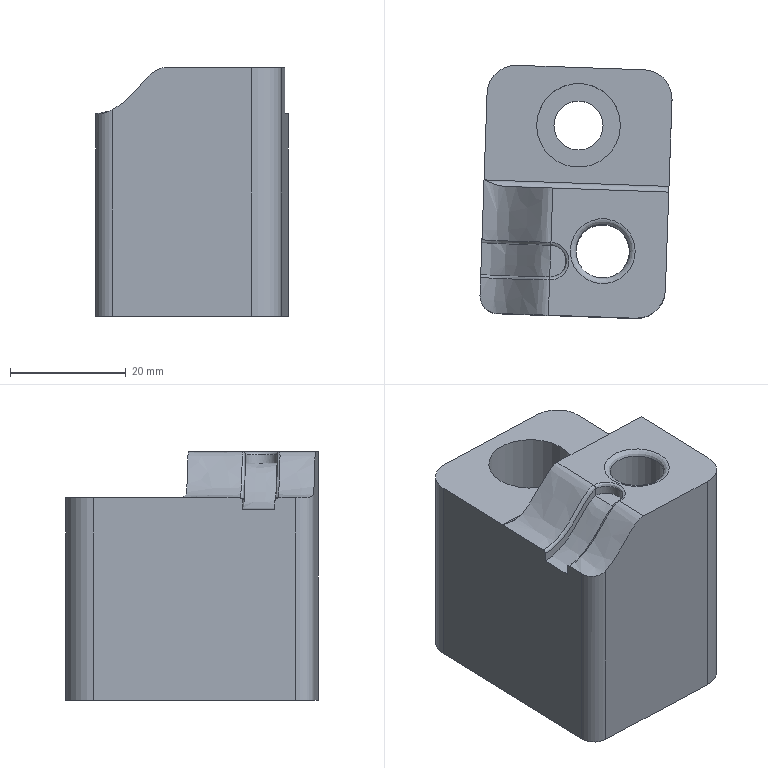Part | NX | features DIE-55 2 | 1 solid | 29 faces | box 33.207 x 43.748 x 43 mm | volume 45246 mm3 | plane 10 | spline 10 | cylinder 8 | torus 1 | commonest cylinder face diameters 10 x3 2 x1 6 x1 8.5 x1 9.27 x1 14.5 x1